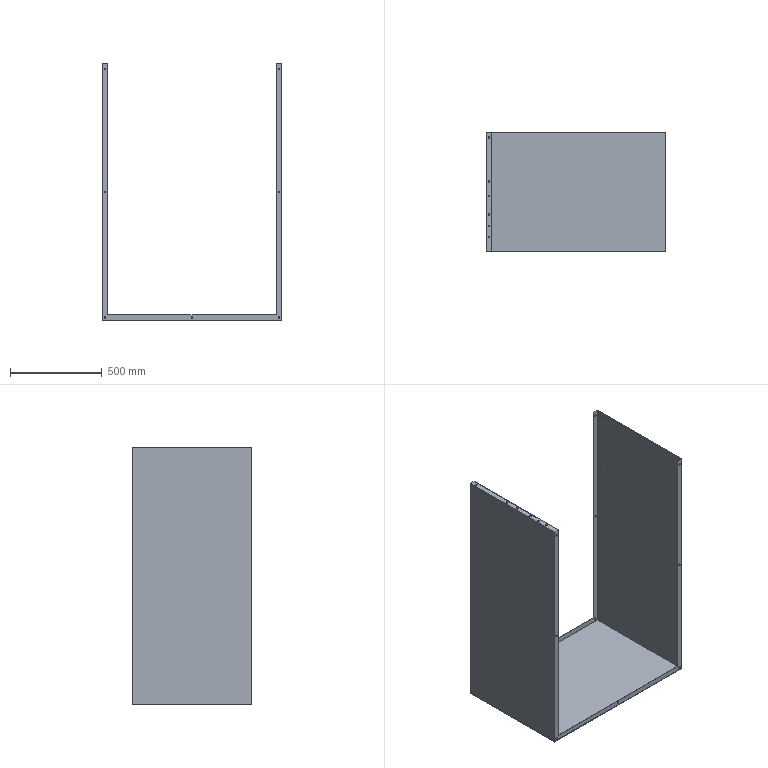Part | SolidWorks | features ICE 6, Extrusion 1 | 1 solid | 70 faces | box 980 x 650 x 1400 mm | volume 5357860 mm3 | cylinder 52 | plane 18 | commonest cylinder face diameters 9 x52